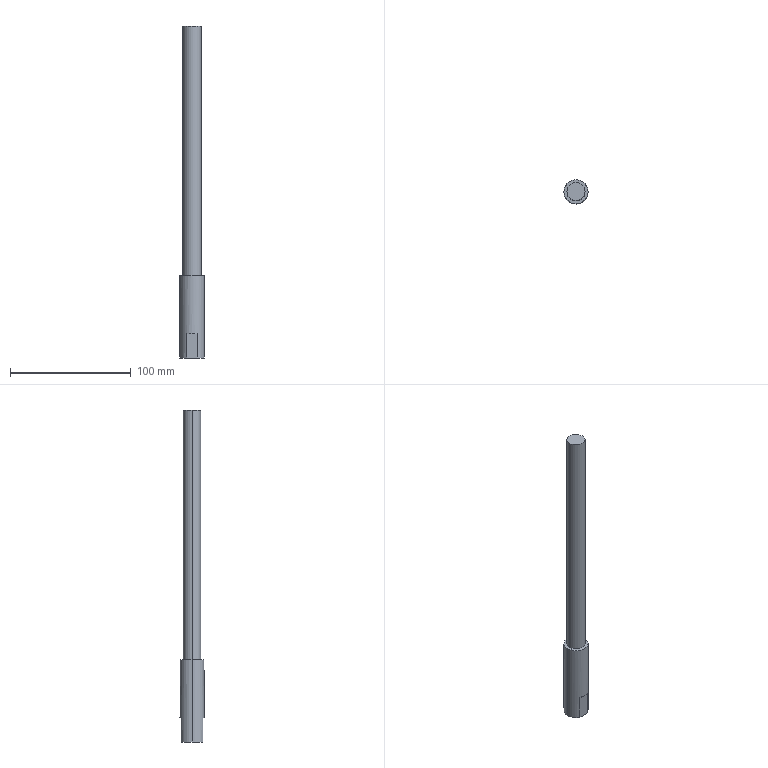Part | SolidWorks | features ICE 2, 3DProfileFeature 1, Extrusion 1, HoleWzd 1 | 1 solid | 17 faces | box 20 x 20 x 275 mm | volume 57016 mm3 | plane 7 | cylinder 6 | cone 4 | commonest cylinder face diameters 6.8 x2 15 x2 20 x2
STEP:
#1=CARTESIAN_POINT('',(3.4,0.,-67.375));
#2=VERTEX_POINT('',#1);
#3=CARTESIAN_POINT('',(-3.4,0.,-67.375));
#4=VERTEX_POINT('',#3);
#5=CARTESIAN_POINT('',(0.,0.,-67.375));
#6=DIRECTION('',(0.,0.,-1.));
#7=DIRECTION('',(-1.,0.,0.));
#8=AXIS2_PLACEMENT_3D('',#5,#6,#7);
#9=CIRCLE('',#8,3.4);
#10=EDGE_CURVE('',#2,#4,#9,.T.);
#11=ORIENTED_EDGE('',*,*,#10,.F.);
#12=CARTESIAN_POINT('',(4.025,0.,-68.));
#13=VERTEX_POINT('',#12);
#14=CARTESIAN_POINT('',(4.025,0.,-68.));
#15=DIRECTION('',(0.7071,0.,-0.7071));
#16=VECTOR('',#15,1000.);
#17=LINE('',#14,#16);
#18=EDGE_CURVE('',#2,#13,#17,.T.);
#19=ORIENTED_EDGE('',*,*,#18,.T.);
#20=CARTESIAN_POINT('',(-4.025,0.,-68.));
#21=VERTEX_POINT('',#20);
#22=CARTESIAN_POINT('',(0.,0.,-68.));
#23=DIRECTION('',(0.,0.,-1.));
#24=DIRECTION('',(-1.,0.,0.));
#25=AXIS2_PLACEMENT_3D('',#22,#23,#24);
#26=CIRCLE('',#25,4.025);
#27=EDGE_CURVE('',#13,#21,#26,.T.);
#28=ORIENTED_EDGE('',*,*,#27,.T.);
#29=CARTESIAN_POINT('',(-4.025,0.,-68.));
#30=DIRECTION('',(-0.7071,0.,-0.7071));
#31=VECTOR('',#30,1000.);
#32=LINE('',#29,#31);
#33=EDGE_CURVE('',#4,#21,#32,.T.);
#34=ORIENTED_EDGE('',*,*,#33,.F.);
#35=EDGE_LOOP('',(#11,#19,#28,#34));
#36=FACE_OUTER_BOUND('',#35,.T.);
#37=CARTESIAN_POINT('',(0.,0.,-68.));
#38=DIRECTION('',(0.,0.,-1.));
#39=DIRECTION('',(-1.,0.,0.));
#40=AXIS2_PLACEMENT_3D('',#37,#38,#39);
#41=CONICAL_SURFACE('',#40,4.025,0.7854);
#42=ADVANCED_FACE('',(#36),#41,.F.);
#43=CARTESIAN_POINT('',(3.4,0.,-49.75));
#44=VERTEX_POINT('',#43);
#45=CARTESIAN_POINT('',(-3.4,0.,-49.75));
#46=VERTEX_POINT('',#45);
#47=CARTESIAN_POINT('',(0.,0.,-49.75));
#48=DIRECTION('',(0.,0.,-1.));
#49=DIRECTION('',(-1.,0.,0.));
#50=AXIS2_PLACEMENT_3D('',#47,#48,#49);
#51=CIRCLE('',#50,3.4);
#52=EDGE_CURVE('',#44,#46,#51,.T.);
#53=ORIENTED_EDGE('',*,*,#52,.F.);
#54=CARTESIAN_POINT('',(3.4,0.,-68.));
#55=DIRECTION('',(0.,0.,-1.));
#56=VECTOR('',#55,1000.);
#57=LINE('',#54,#56);
#58=EDGE_CURVE('',#44,#2,#57,.T.);
#59=ORIENTED_EDGE('',*,*,#58,.T.);
#60=ORIENTED_EDGE('',*,*,#10,.T.);
#61=CARTESIAN_POINT('',(-3.4,0.,-68.));
#62=DIRECTION('',(0.,0.,-1.));
#63=VECTOR('',#62,1000.);
#64=LINE('',#61,#63);
#65=EDGE_CURVE('',#46,#4,#64,.T.);
#66=ORIENTED_EDGE('',*,*,#65,.F.);
#67=EDGE_LOOP('',(#53,#59,#60,#66));
#68=FACE_OUTER_BOUND('',#67,.T.);
#69=CARTESIAN_POINT('',(0.,0.,-68.));
#70=DIRECTION('',(0.,0.,-1.));
#71=DIRECTION('',(-1.,0.,0.));
#72=AXIS2_PLACEMENT_3D('',#69,#70,#71);
#73=CYLINDRICAL_SURFACE('',#72,3.4);
#74=ADVANCED_FACE('',(#68),#73,.F.);
#75=CARTESIAN_POINT('',(0.,0.,-47.707));
#76=VERTEX_POINT('',#75);
#77=CARTESIAN_POINT('',(-3.4,0.,-49.75));
#78=DIRECTION('',(-0.8572,0.,-0.515));
#79=VECTOR('',#78,1000.);
#80=LINE('',#77,#79);
#81=EDGE_CURVE('',#76,#46,#80,.T.);
#82=ORIENTED_EDGE('',*,*,#81,.F.);
#83=CARTESIAN_POINT('',(3.4,0.,-49.75));
#84=DIRECTION('',(0.8572,0.,-0.515));
#85=VECTOR('',#84,1000.);
#86=LINE('',#83,#85);
#87=EDGE_CURVE('',#76,#44,#86,.T.);
#88=ORIENTED_EDGE('',*,*,#87,.T.);
#89=ORIENTED_EDGE('',*,*,#52,.T.);
#90=EDGE_LOOP('',(#82,#88,#89));
#91=FACE_OUTER_BOUND('',#90,.T.);
#92=CARTESIAN_POINT('',(0.,0.,-49.75));
#93=DIRECTION('',(0.,0.,-1.));
#94=DIRECTION('',(-1.,0.,0.));
#95=AXIS2_PLACEMENT_3D('',#92,#93,#94);
#96=CONICAL_SURFACE('',#95,3.4,1.03);
#97=ADVANCED_FACE('',(#91),#96,.F.);
#98=CARTESIAN_POINT('',(7.5,0.,207.));
#99=VERTEX_POINT('',#98);
#100=CARTESIAN_POINT('',(-7.5,0.,207.));
#101=VERTEX_POINT('',#100);
#102=CARTESIAN_POINT('',(0.,0.,207.));
#103=DIRECTION('',(0.,0.,1.));
#104=DIRECTION('',(1.,0.,0.));
#105=AXIS2_PLACEMENT_3D('',#102,#103,#104);
#106=CIRCLE('',#105,7.5);
#107=EDGE_CURVE('',#99,#101,#106,.T.);
#108=ORIENTED_EDGE('',*,*,#107,.F.);
#109=CARTESIAN_POINT('',(7.5,0.,0.));
#110=VERTEX_POINT('',#109);
#111=CARTESIAN_POINT('',(7.5,0.,207.));
#112=DIRECTION('',(0.,0.,-1.));
#113=VECTOR('',#112,1000.);
#114=LINE('',#111,#113);
#115=EDGE_CURVE('',#99,#110,#114,.T.);
#116=ORIENTED_EDGE('',*,*,#115,.T.);
#117=CARTESIAN_POINT('',(-7.5,0.,0.));
#118=VERTEX_POINT('',#117);
#119=CARTESIAN_POINT('',(0.,0.,0.));
#120=DIRECTION('',(0.,0.,1.));
#121=DIRECTION('',(1.,0.,0.));
#122=AXIS2_PLACEMENT_3D('',#119,#120,#121);
#123=CIRCLE('',#122,7.5);
#124=EDGE_CURVE('',#110,#118,#123,.T.);
#125=ORIENTED_EDGE('',*,*,#124,.T.);
#126=CARTESIAN_POINT('',(-7.5,0.,207.));
#127=DIRECTION('',(0.,0.,-1.));
#128=VECTOR('',#127,1000.);
#129=LINE('',#126,#128);
#130=EDGE_CURVE('',#101,#118,#129,.T.);
#131=ORIENTED_EDGE('',*,*,#130,.F.);
#132=EDGE_LOOP('',(#108,#116,#125,#131));
#133=FACE_OUTER_BOUND('',#132,.T.);
#134=CARTESIAN_POINT('',(0.,0.,207.));
#135=DIRECTION('',(0.,0.,-1.));
#136=DIRECTION('',(-1.,0.,0.));
#137=AXIS2_PLACEMENT_3D('',#134,#135,#136);
#138=CYLINDRICAL_SURFACE('',#137,7.5);
#139=ADVANCED_FACE('',(#133),#138,.T.);
#140=CARTESIAN_POINT('',(-10.,0.,-68.));
#141=VERTEX_POINT('',#140);
#142=CARTESIAN_POINT('',(-4.359,9.,-68.));
#143=VERTEX_POINT('',#142);
#144=CARTESIAN_POINT('',(0.,0.,-68.));
#145=DIRECTION('',(0.,0.,-1.));
#146=DIRECTION('',(-1.,0.,0.));
#147=AXIS2_PLACEMENT_3D('',#144,#145,#146);
#148=CIRCLE('',#147,10.);
#149=EDGE_CURVE('',#141,#143,#148,.T.);
#150=ORIENTED_EDGE('',*,*,#149,.F.);
#151=CARTESIAN_POINT('',(-10.,0.,0.));
#152=VERTEX_POINT('',#151);
#153=CARTESIAN_POINT('',(-10.,0.,-68.));
#154=DIRECTION('',(0.,0.,1.));
#155=VECTOR('',#154,1000.);
#156=LINE('',#153,#155);
#157=EDGE_CURVE('',#141,#152,#156,.T.);
#158=ORIENTED_EDGE('',*,*,#157,.T.);
#159=CARTESIAN_POINT('',(10.,0.,0.));
#160=VERTEX_POINT('',#159);
#161=CARTESIAN_POINT('',(0.,0.,0.));
#162=DIRECTION('',(0.,0.,-1.));
#163=DIRECTION('',(-1.,0.,0.));
#164=AXIS2_PLACEMENT_3D('',#161,#162,#163);
#165=CIRCLE('',#164,10.);
#166=EDGE_CURVE('',#152,#160,#165,.T.);
#167=ORIENTED_EDGE('',*,*,#166,.T.);
#168=CARTESIAN_POINT('',(10.,0.,-68.));
#169=VERTEX_POINT('',#168);
#170=CARTESIAN_POINT('',(10.,0.,-68.));
#171=DIRECTION('',(0.,0.,1.));
#172=VECTOR('',#171,1000.);
#173=LINE('',#170,#172);
#174=EDGE_CURVE('',#169,#160,#173,.T.);
#175=ORIENTED_EDGE('',*,*,#174,.F.);
#176=CARTESIAN_POINT('',(4.359,9.,-68.));
#177=VERTEX_POINT('',#176);
#178=CARTESIAN_POINT('',(0.,0.,-68.));
#179=DIRECTION('',(0.,0.,-1.));
#180=DIRECTION('',(-1.,0.,0.));
#181=AXIS2_PLACEMENT_3D('',#178,#179,#180);
#182=CIRCLE('',#181,10.);
#183=EDGE_CURVE('',#177,#169,#182,.T.);
#184=ORIENTED_EDGE('',*,*,#183,.F.);
#185=CARTESIAN_POINT('',(4.359,9.,-48.));
#186=VERTEX_POINT('',#185);
#187=CARTESIAN_POINT('',(4.359,9.,-68.));
#188=DIRECTION('',(0.,0.,-1.));
#189=VECTOR('',#188,1000.);
#190=LINE('',#187,#189);
#191=EDGE_CURVE('',#186,#177,#190,.T.);
#192=ORIENTED_EDGE('',*,*,#191,.F.);
#193=CARTESIAN_POINT('',(-4.359,9.,-48.));
#194=VERTEX_POINT('',#193);
#195=CARTESIAN_POINT('',(0.,0.,-48.));
#196=DIRECTION('',(0.,0.,-1.));
#197=DIRECTION('',(-1.,0.,0.));
#198=AXIS2_PLACEMENT_3D('',#195,#196,#197);
#199=CIRCLE('',#198,10.);
#200=EDGE_CURVE('',#194,#186,#199,.T.);
#201=ORIENTED_EDGE('',*,*,#200,.F.);
#202=CARTESIAN_POINT('',(-4.359,9.,-68.));
#203=DIRECTION('',(0.,0.,1.));
#204=VECTOR('',#203,1000.);
#205=LINE('',#202,#204);
#206=EDGE_CURVE('',#143,#194,#205,.T.);
#207=ORIENTED_EDGE('',*,*,#206,.F.);
#208=EDGE_LOOP('',(#150,#158,#167,#175,#184,#192,#201,#207));
#209=FACE_OUTER_BOUND('',#208,.T.);
#210=CARTESIAN_POINT('',(0.,0.,-68.));
#211=DIRECTION('',(0.,0.,1.));
#212=DIRECTION('',(1.,0.,0.));
#213=AXIS2_PLACEMENT_3D('',#210,#211,#212);
#214=CYLINDRICAL_SURFACE('',#213,10.);
#215=ADVANCED_FACE('',(#209),#214,.T.);
#216=ORIENTED_EDGE('',*,*,#157,.F.);
#217=CARTESIAN_POINT('',(-4.359,-9.,-68.));
#218=VERTEX_POINT('',#217);
#219=CARTESIAN_POINT('',(0.,0.,-68.));
#220=DIRECTION('',(0.,0.,-1.));
#221=DIRECTION('',(-1.,0.,0.));
#222=AXIS2_PLACEMENT_3D('',#219,#220,#221);
#223=CIRCLE('',#222,10.);
#224=EDGE_CURVE('',#218,#141,#223,.T.);
#225=ORIENTED_EDGE('',*,*,#224,.F.);
#226=CARTESIAN_POINT('',(-4.359,-9.,-48.));
#227=VERTEX_POINT('',#226);
#228=CARTESIAN_POINT('',(-4.359,-9.,-68.));
#229=DIRECTION('',(0.,0.,-1.));
#230=VECTOR('',#229,1000.);
#231=LINE('',#228,#230);
#232=EDGE_CURVE('',#227,#218,#231,.T.);
#233=ORIENTED_EDGE('',*,*,#232,.F.);
#234=CARTESIAN_POINT('',(4.359,-9.,-48.));
#235=VERTEX_POINT('',#234);
#236=CARTESIAN_POINT('',(0.,0.,-48.));
#237=DIRECTION('',(0.,0.,-1.));
#238=DIRECTION('',(-1.,0.,0.));
#239=AXIS2_PLACEMENT_3D('',#236,#237,#238);
#240=CIRCLE('',#239,10.);
#241=EDGE_CURVE('',#235,#227,#240,.T.);
#242=ORIENTED_EDGE('',*,*,#241,.F.);
#243=CARTESIAN_POINT('',(4.359,-9.,-68.));
#244=VERTEX_POINT('',#243);
#245=CARTESIAN_POINT('',(4.359,-9.,-68.));
#246=DIRECTION('',(0.,0.,1.));
#247=VECTOR('',#246,1000.);
#248=LINE('',#245,#247);
#249=EDGE_CURVE('',#244,#235,#248,.T.);
#250=ORIENTED_EDGE('',*,*,#249,.F.);
#251=CARTESIAN_POINT('',(0.,0.,-68.));
#252=DIRECTION('',(0.,0.,-1.));
#253=DIRECTION('',(-1.,0.,0.));
#254=AXIS2_PLACEMENT_3D('',#251,#252,#253);
#255=CIRCLE('',#254,10.);
#256=EDGE_CURVE('',#169,#244,#255,.T.);
#257=ORIENTED_EDGE('',*,*,#256,.F.);
#258=ORIENTED_EDGE('',*,*,#174,.T.);
#259=CARTESIAN_POINT('',(0.,0.,0.));
#260=DIRECTION('',(0.,0.,-1.));
#261=DIRECTION('',(-1.,0.,0.));
#262=AXIS2_PLACEMENT_3D('',#259,#260,#261);
#263=CIRCLE('',#262,10.);
#264=EDGE_CURVE('',#160,#152,#263,.T.);
#265=ORIENTED_EDGE('',*,*,#264,.T.);
#266=EDGE_LOOP('',(#216,#225,#233,#242,#250,#257,#258,#265));
#267=FACE_OUTER_BOUND('',#266,.T.);
#268=CARTESIAN_POINT('',(0.,0.,-68.));
#269=DIRECTION('',(0.,0.,1.));
#270=DIRECTION('',(1.,0.,0.));
#271=AXIS2_PLACEMENT_3D('',#268,#269,#270);
#272=CYLINDRICAL_SURFACE('',#271,10.);
#273=ADVANCED_FACE('',(#267),#272,.T.);
#274=CARTESIAN_POINT('',(0.,0.,-68.));
#275=DIRECTION('',(0.,0.,-1.));
#276=DIRECTION('',(-1.,0.,0.));
#277=AXIS2_PLACEMENT_3D('',#274,#275,#276);
#278=CIRCLE('',#277,4.025);
#279=EDGE_CURVE('',#21,#13,#278,.T.);
#280=ORIENTED_EDGE('',*,*,#279,.F.);
#281=ORIENTED_EDGE('',*,*,#27,.F.);
#282=EDGE_LOOP('',(#280,#281));
#283=FACE_BOUND('',#282,.T.);
#284=ORIENTED_EDGE('',*,*,#183,.T.);
#285=ORIENTED_EDGE('',*,*,#256,.T.);
#286=CARTESIAN_POINT('',(0.,-9.,-68.));
#287=DIRECTION('',(-1.,0.,0.));
#288=VECTOR('',#287,1000.);
#289=LINE('',#286,#288);
#290=EDGE_CURVE('',#244,#218,#289,.T.);
#291=ORIENTED_EDGE('',*,*,#290,.T.);
#292=ORIENTED_EDGE('',*,*,#224,.T.);
#293=ORIENTED_EDGE('',*,*,#149,.T.);
#294=CARTESIAN_POINT('',(0.,9.,-68.));
#295=DIRECTION('',(1.,0.,0.));
#296=VECTOR('',#295,1000.);
#297=LINE('',#294,#296);
#298=EDGE_CURVE('',#143,#177,#297,.T.);
#299=ORIENTED_EDGE('',*,*,#298,.T.);
#300=EDGE_LOOP('',(#284,#285,#291,#292,#293,#299));
#301=FACE_OUTER_BOUND('',#300,.T.);
#302=CARTESIAN_POINT('',(0.,0.,-68.));
#303=DIRECTION('',(0.,0.,-1.));
#304=DIRECTION('',(-1.,0.,0.));
#305=AXIS2_PLACEMENT_3D('',#302,#303,#304);
#306=PLANE('',#305);
#307=ADVANCED_FACE('',(#283,#301),#306,.T.);
#308=ORIENTED_EDGE('',*,*,#115,.F.);
#309=CARTESIAN_POINT('',(0.,0.,207.));
#310=DIRECTION('',(0.,0.,1.));
#311=DIRECTION('',(1.,0.,0.));
#312=AXIS2_PLACEMENT_3D('',#309,#310,#311);
#313=CIRCLE('',#312,7.5);
#314=EDGE_CURVE('',#101,#99,#313,.T.);
#315=ORIENTED_EDGE('',*,*,#314,.F.);
#316=ORIENTED_EDGE('',*,*,#130,.T.);
#317=CARTESIAN_POINT('',(0.,0.,0.));
#318=DIRECTION('',(0.,0.,1.));
#319=DIRECTION('',(1.,0.,0.));
#320=AXIS2_PLACEMENT_3D('',#317,#318,#319);
#321=CIRCLE('',#320,7.5);
#322=EDGE_CURVE('',#118,#110,#321,.T.);
#323=ORIENTED_EDGE('',*,*,#322,.T.);
#324=EDGE_LOOP('',(#308,#315,#316,#323));
#325=FACE_OUTER_BOUND('',#324,.T.);
#326=CARTESIAN_POINT('',(0.,0.,207.));
#327=DIRECTION('',(0.,0.,-1.));
#328=DIRECTION('',(-1.,0.,0.));
#329=AXIS2_PLACEMENT_3D('',#326,#327,#328);
#330=CYLINDRICAL_SURFACE('',#329,7.5);
#331=ADVANCED_FACE('',(#325),#330,.T.);
#332=ORIENTED_EDGE('',*,*,#314,.T.);
#333=ORIENTED_EDGE('',*,*,#107,.T.);
#334=EDGE_LOOP('',(#332,#333));
#335=FACE_OUTER_BOUND('',#334,.T.);
#336=CARTESIAN_POINT('',(0.,0.,207.));
#337=DIRECTION('',(0.,0.,1.));
#338=DIRECTION('',(1.,0.,0.));
#339=AXIS2_PLACEMENT_3D('',#336,#337,#338);
#340=PLANE('',#339);
#341=ADVANCED_FACE('',(#335),#340,.T.);
#342=ORIENTED_EDGE('',*,*,#322,.F.);
#343=ORIENTED_EDGE('',*,*,#124,.F.);
#344=EDGE_LOOP('',(#342,#343));
#345=FACE_BOUND('',#344,.T.);
#346=ORIENTED_EDGE('',*,*,#264,.F.);
#347=ORIENTED_EDGE('',*,*,#166,.F.);
#348=EDGE_LOOP('',(#346,#347));
#349=FACE_OUTER_BOUND('',#348,.T.);
#350=CARTESIAN_POINT('',(0.,0.,0.));
#351=DIRECTION('',(0.,0.,-1.));
#352=DIRECTION('',(-1.,0.,0.));
#353=AXIS2_PLACEMENT_3D('',#350,#351,#352);
#354=PLANE('',#353);
#355=ADVANCED_FACE('',(#345,#349),#354,.F.);
#356=ORIENTED_EDGE('',*,*,#206,.T.);
#357=CARTESIAN_POINT('',(11.5,9.,-48.));
#358=DIRECTION('',(1.,0.,0.));
#359=VECTOR('',#358,1000.);
#360=LINE('',#357,#359);
#361=EDGE_CURVE('',#194,#186,#360,.T.);
#362=ORIENTED_EDGE('',*,*,#361,.T.);
#363=ORIENTED_EDGE('',*,*,#191,.T.);
#364=ORIENTED_EDGE('',*,*,#298,.F.);
#365=EDGE_LOOP('',(#356,#362,#363,#364));
#366=FACE_OUTER_BOUND('',#365,.T.);
#367=CARTESIAN_POINT('',(11.5,9.,-48.));
#368=DIRECTION('',(0.,1.,0.));
#369=DIRECTION('',(0.,0.,1.));
#370=AXIS2_PLACEMENT_3D('',#367,#368,#369);
#371=PLANE('',#370);
#372=ADVANCED_FACE('',(#366),#371,.T.);
#373=ORIENTED_EDGE('',*,*,#200,.T.);
#374=ORIENTED_EDGE('',*,*,#361,.F.);
#375=EDGE_LOOP('',(#373,#374));
#376=FACE_OUTER_BOUND('',#375,.T.);
#377=CARTESIAN_POINT('',(0.,0.,-48.));
#378=DIRECTION('',(0.,0.,-1.));
#379=DIRECTION('',(-1.,0.,0.));
#380=AXIS2_PLACEMENT_3D('',#377,#378,#379);
#381=PLANE('',#380);
#382=ADVANCED_FACE('',(#376),#381,.T.);
#383=ORIENTED_EDGE('',*,*,#241,.T.);
#384=CARTESIAN_POINT('',(11.5,-9.,-48.));
#385=DIRECTION('',(-1.,0.,0.));
#386=VECTOR('',#385,1000.);
#387=LINE('',#384,#386);
#388=EDGE_CURVE('',#235,#227,#387,.T.);
#389=ORIENTED_EDGE('',*,*,#388,.F.);
#390=EDGE_LOOP('',(#383,#389));
#391=FACE_OUTER_BOUND('',#390,.T.);
#392=CARTESIAN_POINT('',(0.,0.,-48.));
#393=DIRECTION('',(0.,0.,-1.));
#394=DIRECTION('',(-1.,0.,0.));
#395=AXIS2_PLACEMENT_3D('',#392,#393,#394);
#396=PLANE('',#395);
#397=ADVANCED_FACE('',(#391),#396,.T.);
#398=ORIENTED_EDGE('',*,*,#249,.T.);
#399=ORIENTED_EDGE('',*,*,#388,.T.);
#400=ORIENTED_EDGE('',*,*,#232,.T.);
#401=ORIENTED_EDGE('',*,*,#290,.F.);
#402=EDGE_LOOP('',(#398,#399,#400,#401));
#403=FACE_OUTER_BOUND('',#402,.T.);
#404=CARTESIAN_POINT('',(11.5,-9.,-48.));
#405=DIRECTION('',(0.,-1.,0.));
#406=DIRECTION('',(0.,0.,-1.));
#407=AXIS2_PLACEMENT_3D('',#404,#405,#406);
#408=PLANE('',#407);
#409=ADVANCED_FACE('',(#403),#408,.T.);
#410=ORIENTED_EDGE('',*,*,#87,.F.);
#411=ORIENTED_EDGE('',*,*,#81,.T.);
#412=CARTESIAN_POINT('',(0.,0.,-49.75));
#413=DIRECTION('',(0.,0.,-1.));
#414=DIRECTION('',(-1.,0.,0.));
#415=AXIS2_PLACEMENT_3D('',#412,#413,#414);
#416=CIRCLE('',#415,3.4);
#417=EDGE_CURVE('',#46,#44,#416,.T.);
#418=ORIENTED_EDGE('',*,*,#417,.T.);
#419=EDGE_LOOP('',(#410,#411,#418));
#420=FACE_OUTER_BOUND('',#419,.T.);
#421=CARTESIAN_POINT('',(0.,0.,-49.75));
#422=DIRECTION('',(0.,0.,-1.));
#423=DIRECTION('',(-1.,0.,0.));
#424=AXIS2_PLACEMENT_3D('',#421,#422,#423);
#425=CONICAL_SURFACE('',#424,3.4,1.03);
#426=ADVANCED_FACE('',(#420),#425,.F.);
#427=ORIENTED_EDGE('',*,*,#58,.F.);
#428=ORIENTED_EDGE('',*,*,#417,.F.);
#429=ORIENTED_EDGE('',*,*,#65,.T.);
#430=CARTESIAN_POINT('',(0.,0.,-67.375));
#431=DIRECTION('',(0.,0.,-1.));
#432=DIRECTION('',(-1.,0.,0.));
#433=AXIS2_PLACEMENT_3D('',#430,#431,#432);
#434=CIRCLE('',#433,3.4);
#435=EDGE_CURVE('',#4,#2,#434,.T.);
#436=ORIENTED_EDGE('',*,*,#435,.T.);
#437=EDGE_LOOP('',(#427,#428,#429,#436));
#438=FACE_OUTER_BOUND('',#437,.T.);
#439=CARTESIAN_POINT('',(0.,0.,-68.));
#440=DIRECTION('',(0.,0.,-1.));
#441=DIRECTION('',(-1.,0.,0.));
#442=AXIS2_PLACEMENT_3D('',#439,#440,#441);
#443=CYLINDRICAL_SURFACE('',#442,3.4);
#444=ADVANCED_FACE('',(#438),#443,.F.);
#445=ORIENTED_EDGE('',*,*,#18,.F.);
#446=ORIENTED_EDGE('',*,*,#435,.F.);
#447=ORIENTED_EDGE('',*,*,#33,.T.);
#448=ORIENTED_EDGE('',*,*,#279,.T.);
#449=EDGE_LOOP('',(#445,#446,#447,#448));
#450=FACE_OUTER_BOUND('',#449,.T.);
#451=CARTESIAN_POINT('',(0.,0.,-68.));
#452=DIRECTION('',(0.,0.,-1.));
#453=DIRECTION('',(-1.,0.,0.));
#454=AXIS2_PLACEMENT_3D('',#451,#452,#453);
#455=CONICAL_SURFACE('',#454,4.025,0.7854);
#456=ADVANCED_FACE('',(#450),#455,.F.);
#457=CLOSED_SHELL('',(#42,#74,#97,#139,#215,#273,#307,#331,#341,#355,#372,#382,#397,#409,#426,#444,#456));
#458=MANIFOLD_SOLID_BREP('',#457);
#459=CARTESIAN_POINT('',(0.,0.,0.));
#460=DIRECTION('',(0.,0.,1.));
#461=DIRECTION('',(1.,0.,0.));
#462=AXIS2_PLACEMENT_3D('',#459,#460,#461);
#463=(LENGTH_UNIT()NAMED_UNIT(*)SI_UNIT(.MILLI.,.METRE.));
#464=UNCERTAINTY_MEASURE_WITH_UNIT(LENGTH_MEASURE(0.00001),#463,'','');
#465=(NAMED_UNIT(*)PLANE_ANGLE_UNIT()SI_UNIT($,.RADIAN.));
#466=(NAMED_UNIT(*)SI_UNIT($,.STERADIAN.)SOLID_ANGLE_UNIT());
#467=(GEOMETRIC_REPRESENTATION_CONTEXT(3)GLOBAL_UNCERTAINTY_ASSIGNED_CONTEXT((#464))GLOBAL_UNIT_ASSIGNED_CONTEXT((#463,#465,#466))REPRESENTATION_CONTEXT('',''));
#468=ADVANCED_BREP_SHAPE_REPRESENTATION('',(#458,#462),#467);